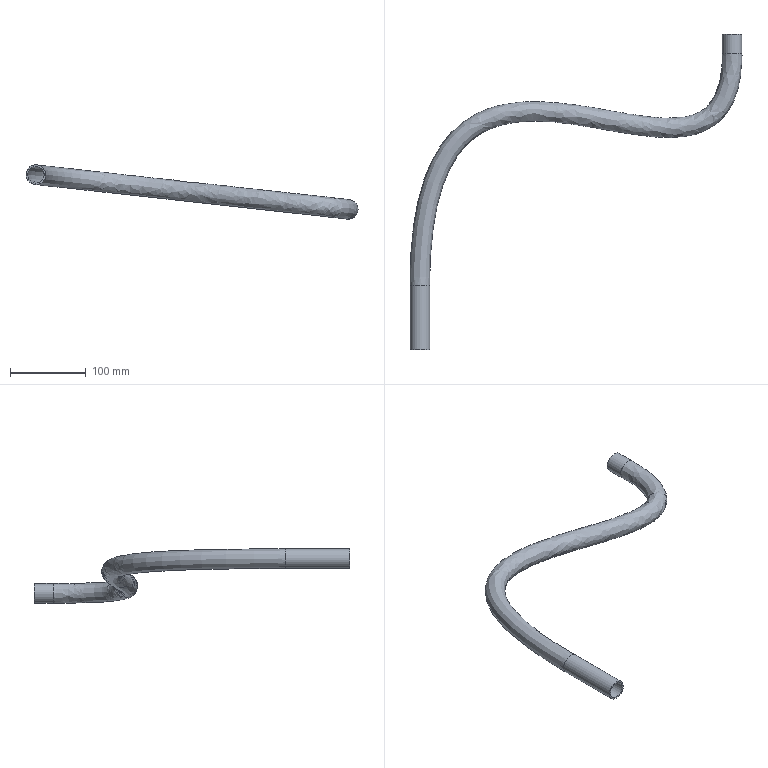Part | STEP file | Part 6^JBJ-F-0000-00 | 1 solid | 8 faces | box 437.091 x 414.992 x 71.5 mm | volume 113332 mm3 | cylinder 4 | spline 2 | plane 2 | commonest cylinder face diameters 22 x2 26 x2